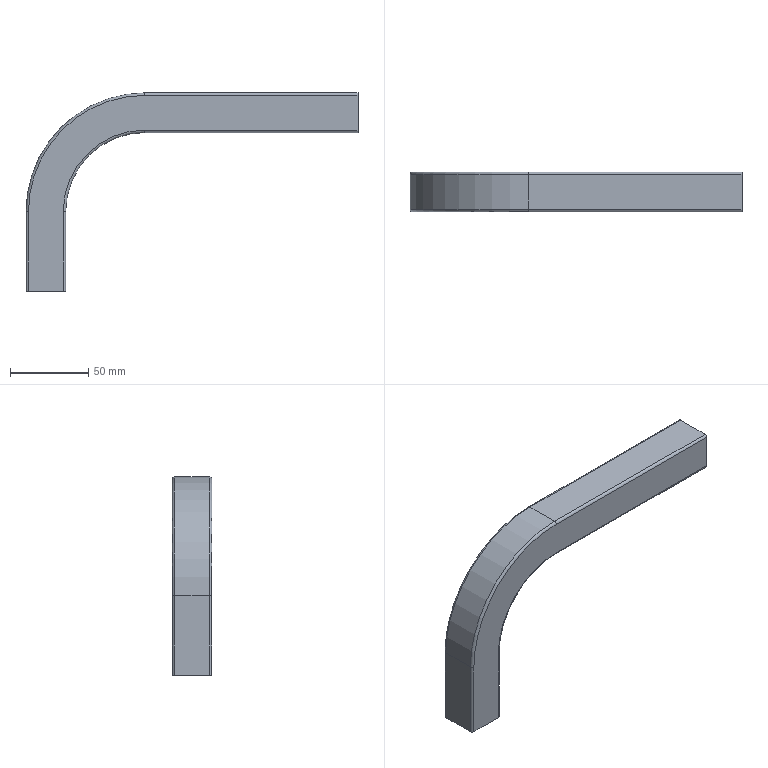Part | NX | features BREP 1 | 1 solid | 30 faces | box 212.725 x 25.4 x 127 mm | volume 52656 mm3 | plane 14 | cylinder 12 | torus 4 | commonest cylinder face diameters 3.175 x8 101.6 x1 105.562 x1 148.438 x1 152.4 x1
STEP:
#1=CARTESIAN_POINT('',(11.113,12.7,-114.3));
#2=VERTEX_POINT('',#1);
#3=CARTESIAN_POINT('',(-11.113,12.7,-114.3));
#4=VERTEX_POINT('',#3);
#5=CARTESIAN_POINT('',(11.113,12.7,-114.3));
#6=DIRECTION('',(-1.,0.,0.));
#7=VECTOR('',#6,1000.);
#8=LINE('',#5,#7);
#9=EDGE_CURVE('',#2,#4,#8,.T.);
#10=ORIENTED_EDGE('',*,*,#9,.F.);
#11=CARTESIAN_POINT('',(12.7,11.113,-114.3));
#12=VERTEX_POINT('',#11);
#13=CARTESIAN_POINT('',(11.113,11.113,-114.3));
#14=DIRECTION('',(0.,0.,-1.));
#15=DIRECTION('',(0.,1.,0.));
#16=AXIS2_PLACEMENT_3D('',#13,#14,#15);
#17=CIRCLE('',#16,1.587);
#18=EDGE_CURVE('',#2,#12,#17,.T.);
#19=ORIENTED_EDGE('',*,*,#18,.T.);
#20=CARTESIAN_POINT('',(12.7,-11.113,-114.3));
#21=VERTEX_POINT('',#20);
#22=CARTESIAN_POINT('',(12.7,-11.113,-114.3));
#23=DIRECTION('',(0.,1.,0.));
#24=VECTOR('',#23,1000.);
#25=LINE('',#22,#24);
#26=EDGE_CURVE('',#21,#12,#25,.T.);
#27=ORIENTED_EDGE('',*,*,#26,.F.);
#28=CARTESIAN_POINT('',(11.113,-12.7,-114.3));
#29=VERTEX_POINT('',#28);
#30=CARTESIAN_POINT('',(11.113,-11.113,-114.3));
#31=DIRECTION('',(0.,0.,-1.));
#32=DIRECTION('',(1.,0.,0.));
#33=AXIS2_PLACEMENT_3D('',#30,#31,#32);
#34=CIRCLE('',#33,1.587);
#35=EDGE_CURVE('',#21,#29,#34,.T.);
#36=ORIENTED_EDGE('',*,*,#35,.T.);
#37=CARTESIAN_POINT('',(-11.113,-12.7,-114.3));
#38=VERTEX_POINT('',#37);
#39=CARTESIAN_POINT('',(-11.113,-12.7,-114.3));
#40=DIRECTION('',(1.,0.,0.));
#41=VECTOR('',#40,1000.);
#42=LINE('',#39,#41);
#43=EDGE_CURVE('',#38,#29,#42,.T.);
#44=ORIENTED_EDGE('',*,*,#43,.F.);
#45=CARTESIAN_POINT('',(-12.7,-11.113,-114.3));
#46=VERTEX_POINT('',#45);
#47=CARTESIAN_POINT('',(-11.113,-11.113,-114.3));
#48=DIRECTION('',(0.,0.,-1.));
#49=DIRECTION('',(0.,-1.,0.));
#50=AXIS2_PLACEMENT_3D('',#47,#48,#49);
#51=CIRCLE('',#50,1.587);
#52=EDGE_CURVE('',#38,#46,#51,.T.);
#53=ORIENTED_EDGE('',*,*,#52,.T.);
#54=CARTESIAN_POINT('',(-12.7,11.113,-114.3));
#55=VERTEX_POINT('',#54);
#56=CARTESIAN_POINT('',(-12.7,11.113,-114.3));
#57=DIRECTION('',(0.,-1.,0.));
#58=VECTOR('',#57,1000.);
#59=LINE('',#56,#58);
#60=EDGE_CURVE('',#55,#46,#59,.T.);
#61=ORIENTED_EDGE('',*,*,#60,.F.);
#62=CARTESIAN_POINT('',(-11.113,11.113,-114.3));
#63=DIRECTION('',(0.,0.,-1.));
#64=DIRECTION('',(-1.,0.,0.));
#65=AXIS2_PLACEMENT_3D('',#62,#63,#64);
#66=CIRCLE('',#65,1.587);
#67=EDGE_CURVE('',#55,#4,#66,.T.);
#68=ORIENTED_EDGE('',*,*,#67,.T.);
#69=EDGE_LOOP('',(#10,#19,#27,#36,#44,#53,#61,#68));
#70=FACE_BOUND('',#69,.T.);
#71=CARTESIAN_POINT('',(-10.719,-10.719,-114.3));
#72=VERTEX_POINT('',#71);
#73=CARTESIAN_POINT('',(-10.719,10.719,-114.3));
#74=VERTEX_POINT('',#73);
#75=CARTESIAN_POINT('',(-10.719,-10.719,-114.3));
#76=DIRECTION('',(0.,1.,0.));
#77=VECTOR('',#76,1000.);
#78=LINE('',#75,#77);
#79=EDGE_CURVE('',#72,#74,#78,.T.);
#80=ORIENTED_EDGE('',*,*,#79,.F.);
#81=CARTESIAN_POINT('',(10.719,-10.719,-114.3));
#82=VERTEX_POINT('',#81);
#83=CARTESIAN_POINT('',(10.719,-10.719,-114.3));
#84=DIRECTION('',(-1.,0.,0.));
#85=VECTOR('',#84,1000.);
#86=LINE('',#83,#85);
#87=EDGE_CURVE('',#82,#72,#86,.T.);
#88=ORIENTED_EDGE('',*,*,#87,.F.);
#89=CARTESIAN_POINT('',(10.719,10.719,-114.3));
#90=VERTEX_POINT('',#89);
#91=CARTESIAN_POINT('',(10.719,10.719,-114.3));
#92=DIRECTION('',(0.,-1.,0.));
#93=VECTOR('',#92,1000.);
#94=LINE('',#91,#93);
#95=EDGE_CURVE('',#90,#82,#94,.T.);
#96=ORIENTED_EDGE('',*,*,#95,.F.);
#97=CARTESIAN_POINT('',(-10.719,10.719,-114.3));
#98=DIRECTION('',(1.,0.,0.));
#99=VECTOR('',#98,1000.);
#100=LINE('',#97,#99);
#101=EDGE_CURVE('',#74,#90,#100,.T.);
#102=ORIENTED_EDGE('',*,*,#101,.F.);
#103=EDGE_LOOP('',(#80,#88,#96,#102));
#104=FACE_BOUND('',#103,.T.);
#105=CARTESIAN_POINT('',(0.,0.,-114.3));
#106=DIRECTION('',(0.,0.,1.));
#107=DIRECTION('',(1.,0.,0.));
#108=AXIS2_PLACEMENT_3D('',#105,#106,#107);
#109=PLANE('',#108);
#110=ADVANCED_FACE('',(#70,#104),#109,.F.);
#111=CARTESIAN_POINT('',(10.719,10.719,-63.5));
#112=VERTEX_POINT('',#111);
#113=CARTESIAN_POINT('',(10.719,10.719,-114.3));
#114=DIRECTION('',(0.,0.,1.));
#115=VECTOR('',#114,1000.);
#116=LINE('',#113,#115);
#117=EDGE_CURVE('',#90,#112,#116,.T.);
#118=ORIENTED_EDGE('',*,*,#117,.T.);
#119=CARTESIAN_POINT('',(63.5,10.719,-10.719));
#120=VERTEX_POINT('',#119);
#121=CARTESIAN_POINT('',(63.5,10.719,-63.5));
#122=DIRECTION('',(0.,1.,0.));
#123=DIRECTION('',(-1.,0.,0.));
#124=AXIS2_PLACEMENT_3D('',#121,#122,#123);
#125=CIRCLE('',#124,52.781);
#126=EDGE_CURVE('',#112,#120,#125,.T.);
#127=ORIENTED_EDGE('',*,*,#126,.T.);
#128=CARTESIAN_POINT('',(200.025,10.719,-10.719));
#129=VERTEX_POINT('',#128);
#130=CARTESIAN_POINT('',(63.5,10.719,-10.719));
#131=DIRECTION('',(1.,0.,0.));
#132=VECTOR('',#131,1000.);
#133=LINE('',#130,#132);
#134=EDGE_CURVE('',#120,#129,#133,.T.);
#135=ORIENTED_EDGE('',*,*,#134,.T.);
#136=CARTESIAN_POINT('',(200.025,10.719,10.719));
#137=VERTEX_POINT('',#136);
#138=CARTESIAN_POINT('',(200.025,10.719,10.719));
#139=DIRECTION('',(0.,0.,-1.));
#140=VECTOR('',#139,1000.);
#141=LINE('',#138,#140);
#142=EDGE_CURVE('',#137,#129,#141,.T.);
#143=ORIENTED_EDGE('',*,*,#142,.F.);
#144=CARTESIAN_POINT('',(63.5,10.719,10.719));
#145=VERTEX_POINT('',#144);
#146=CARTESIAN_POINT('',(63.5,10.719,10.719));
#147=DIRECTION('',(1.,0.,0.));
#148=VECTOR('',#147,1000.);
#149=LINE('',#146,#148);
#150=EDGE_CURVE('',#145,#137,#149,.T.);
#151=ORIENTED_EDGE('',*,*,#150,.F.);
#152=CARTESIAN_POINT('',(-10.719,10.719,-63.5));
#153=VERTEX_POINT('',#152);
#154=CARTESIAN_POINT('',(63.5,10.719,-63.5));
#155=DIRECTION('',(0.,1.,0.));
#156=DIRECTION('',(-1.,0.,0.));
#157=AXIS2_PLACEMENT_3D('',#154,#155,#156);
#158=CIRCLE('',#157,74.219);
#159=EDGE_CURVE('',#153,#145,#158,.T.);
#160=ORIENTED_EDGE('',*,*,#159,.F.);
#161=CARTESIAN_POINT('',(-10.719,10.719,-114.3));
#162=DIRECTION('',(0.,0.,1.));
#163=VECTOR('',#162,1000.);
#164=LINE('',#161,#163);
#165=EDGE_CURVE('',#74,#153,#164,.T.);
#166=ORIENTED_EDGE('',*,*,#165,.F.);
#167=ORIENTED_EDGE('',*,*,#101,.T.);
#168=EDGE_LOOP('',(#118,#127,#135,#143,#151,#160,#166,#167));
#169=FACE_BOUND('',#168,.T.);
#170=CARTESIAN_POINT('',(-10.719,10.719,-114.3));
#171=DIRECTION('',(0.,-1.,0.));
#172=DIRECTION('',(0.,0.,-1.));
#173=AXIS2_PLACEMENT_3D('',#170,#171,#172);
#174=PLANE('',#173);
#175=ADVANCED_FACE('',(#169),#174,.T.);
#176=ORIENTED_EDGE('',*,*,#165,.T.);
#177=CARTESIAN_POINT('',(-10.719,-10.719,-63.5));
#178=VERTEX_POINT('',#177);
#179=CARTESIAN_POINT('',(-10.719,-10.719,-63.5));
#180=DIRECTION('',(0.,1.,0.));
#181=VECTOR('',#180,1000.);
#182=LINE('',#179,#181);
#183=EDGE_CURVE('',#178,#153,#182,.T.);
#184=ORIENTED_EDGE('',*,*,#183,.F.);
#185=CARTESIAN_POINT('',(-10.719,-10.719,-114.3));
#186=DIRECTION('',(0.,0.,1.));
#187=VECTOR('',#186,1000.);
#188=LINE('',#185,#187);
#189=EDGE_CURVE('',#72,#178,#188,.T.);
#190=ORIENTED_EDGE('',*,*,#189,.F.);
#191=ORIENTED_EDGE('',*,*,#79,.T.);
#192=EDGE_LOOP('',(#176,#184,#190,#191));
#193=FACE_BOUND('',#192,.T.);
#194=CARTESIAN_POINT('',(-10.719,-10.719,-114.3));
#195=DIRECTION('',(1.,0.,0.));
#196=DIRECTION('',(0.,1.,0.));
#197=AXIS2_PLACEMENT_3D('',#194,#195,#196);
#198=PLANE('',#197);
#199=ADVANCED_FACE('',(#193),#198,.T.);
#200=ORIENTED_EDGE('',*,*,#189,.T.);
#201=CARTESIAN_POINT('',(63.5,-10.719,10.719));
#202=VERTEX_POINT('',#201);
#203=CARTESIAN_POINT('',(63.5,-10.719,-63.5));
#204=DIRECTION('',(0.,1.,0.));
#205=DIRECTION('',(-1.,0.,0.));
#206=AXIS2_PLACEMENT_3D('',#203,#204,#205);
#207=CIRCLE('',#206,74.219);
#208=EDGE_CURVE('',#178,#202,#207,.T.);
#209=ORIENTED_EDGE('',*,*,#208,.T.);
#210=CARTESIAN_POINT('',(200.025,-10.719,10.719));
#211=VERTEX_POINT('',#210);
#212=CARTESIAN_POINT('',(63.5,-10.719,10.719));
#213=DIRECTION('',(1.,0.,0.));
#214=VECTOR('',#213,1000.);
#215=LINE('',#212,#214);
#216=EDGE_CURVE('',#202,#211,#215,.T.);
#217=ORIENTED_EDGE('',*,*,#216,.T.);
#218=CARTESIAN_POINT('',(200.025,-10.719,-10.719));
#219=VERTEX_POINT('',#218);
#220=CARTESIAN_POINT('',(200.025,-10.719,-10.719));
#221=DIRECTION('',(0.,0.,1.));
#222=VECTOR('',#221,1000.);
#223=LINE('',#220,#222);
#224=EDGE_CURVE('',#219,#211,#223,.T.);
#225=ORIENTED_EDGE('',*,*,#224,.F.);
#226=CARTESIAN_POINT('',(63.5,-10.719,-10.719));
#227=VERTEX_POINT('',#226);
#228=CARTESIAN_POINT('',(63.5,-10.719,-10.719));
#229=DIRECTION('',(1.,0.,0.));
#230=VECTOR('',#229,1000.);
#231=LINE('',#228,#230);
#232=EDGE_CURVE('',#227,#219,#231,.T.);
#233=ORIENTED_EDGE('',*,*,#232,.F.);
#234=CARTESIAN_POINT('',(10.719,-10.719,-63.5));
#235=VERTEX_POINT('',#234);
#236=CARTESIAN_POINT('',(63.5,-10.719,-63.5));
#237=DIRECTION('',(0.,1.,0.));
#238=DIRECTION('',(-1.,0.,0.));
#239=AXIS2_PLACEMENT_3D('',#236,#237,#238);
#240=CIRCLE('',#239,52.781);
#241=EDGE_CURVE('',#235,#227,#240,.T.);
#242=ORIENTED_EDGE('',*,*,#241,.F.);
#243=CARTESIAN_POINT('',(10.719,-10.719,-114.3));
#244=DIRECTION('',(0.,0.,1.));
#245=VECTOR('',#244,1000.);
#246=LINE('',#243,#245);
#247=EDGE_CURVE('',#82,#235,#246,.T.);
#248=ORIENTED_EDGE('',*,*,#247,.F.);
#249=ORIENTED_EDGE('',*,*,#87,.T.);
#250=EDGE_LOOP('',(#200,#209,#217,#225,#233,#242,#248,#249));
#251=FACE_BOUND('',#250,.T.);
#252=CARTESIAN_POINT('',(10.719,-10.719,-114.3));
#253=DIRECTION('',(0.,1.,0.));
#254=DIRECTION('',(1.,0.,0.));
#255=AXIS2_PLACEMENT_3D('',#252,#253,#254);
#256=PLANE('',#255);
#257=ADVANCED_FACE('',(#251),#256,.T.);
#258=ORIENTED_EDGE('',*,*,#247,.T.);
#259=CARTESIAN_POINT('',(10.719,10.719,-63.5));
#260=DIRECTION('',(0.,-1.,0.));
#261=VECTOR('',#260,1000.);
#262=LINE('',#259,#261);
#263=EDGE_CURVE('',#112,#235,#262,.T.);
#264=ORIENTED_EDGE('',*,*,#263,.F.);
#265=ORIENTED_EDGE('',*,*,#117,.F.);
#266=ORIENTED_EDGE('',*,*,#95,.T.);
#267=EDGE_LOOP('',(#258,#264,#265,#266));
#268=FACE_BOUND('',#267,.T.);
#269=CARTESIAN_POINT('',(10.719,10.719,-114.3));
#270=DIRECTION('',(-1.,0.,0.));
#271=DIRECTION('',(0.,0.,1.));
#272=AXIS2_PLACEMENT_3D('',#269,#270,#271);
#273=PLANE('',#272);
#274=ADVANCED_FACE('',(#268),#273,.T.);
#275=ORIENTED_EDGE('',*,*,#241,.T.);
#276=CARTESIAN_POINT('',(63.5,10.719,-10.719));
#277=DIRECTION('',(0.,-1.,0.));
#278=VECTOR('',#277,1000.);
#279=LINE('',#276,#278);
#280=EDGE_CURVE('',#120,#227,#279,.T.);
#281=ORIENTED_EDGE('',*,*,#280,.F.);
#282=ORIENTED_EDGE('',*,*,#126,.F.);
#283=ORIENTED_EDGE('',*,*,#263,.T.);
#284=EDGE_LOOP('',(#275,#281,#282,#283));
#285=FACE_BOUND('',#284,.T.);
#286=CARTESIAN_POINT('',(63.5,-25.4,-63.5));
#287=DIRECTION('',(0.,1.,0.));
#288=DIRECTION('',(1.,0.,0.));
#289=AXIS2_PLACEMENT_3D('',#286,#287,#288);
#290=CYLINDRICAL_SURFACE('',#289,52.781);
#291=ADVANCED_FACE('',(#285),#290,.T.);
#292=ORIENTED_EDGE('',*,*,#232,.T.);
#293=CARTESIAN_POINT('',(200.025,10.719,-10.719));
#294=DIRECTION('',(0.,-1.,0.));
#295=VECTOR('',#294,1000.);
#296=LINE('',#293,#295);
#297=EDGE_CURVE('',#129,#219,#296,.T.);
#298=ORIENTED_EDGE('',*,*,#297,.F.);
#299=ORIENTED_EDGE('',*,*,#134,.F.);
#300=ORIENTED_EDGE('',*,*,#280,.T.);
#301=EDGE_LOOP('',(#292,#298,#299,#300));
#302=FACE_BOUND('',#301,.T.);
#303=CARTESIAN_POINT('',(63.5,10.719,-10.719));
#304=DIRECTION('',(0.,0.,1.));
#305=DIRECTION('',(1.,0.,0.));
#306=AXIS2_PLACEMENT_3D('',#303,#304,#305);
#307=PLANE('',#306);
#308=ADVANCED_FACE('',(#302),#307,.T.);
#309=CARTESIAN_POINT('',(200.025,11.113,12.7));
#310=VERTEX_POINT('',#309);
#311=CARTESIAN_POINT('',(200.025,-11.113,12.7));
#312=VERTEX_POINT('',#311);
#313=CARTESIAN_POINT('',(200.025,11.113,12.7));
#314=DIRECTION('',(0.,-1.,0.));
#315=VECTOR('',#314,1000.);
#316=LINE('',#313,#315);
#317=EDGE_CURVE('',#310,#312,#316,.T.);
#318=ORIENTED_EDGE('',*,*,#317,.T.);
#319=CARTESIAN_POINT('',(200.025,-12.7,11.113));
#320=VERTEX_POINT('',#319);
#321=CARTESIAN_POINT('',(200.025,-11.113,11.113));
#322=DIRECTION('',(1.,0.,0.));
#323=DIRECTION('',(0.,0.,1.));
#324=AXIS2_PLACEMENT_3D('',#321,#322,#323);
#325=CIRCLE('',#324,1.587);
#326=EDGE_CURVE('',#312,#320,#325,.T.);
#327=ORIENTED_EDGE('',*,*,#326,.T.);
#328=CARTESIAN_POINT('',(200.025,-12.7,-11.113));
#329=VERTEX_POINT('',#328);
#330=CARTESIAN_POINT('',(200.025,-12.7,11.113));
#331=DIRECTION('',(0.,0.,-1.));
#332=VECTOR('',#331,1000.);
#333=LINE('',#330,#332);
#334=EDGE_CURVE('',#320,#329,#333,.T.);
#335=ORIENTED_EDGE('',*,*,#334,.T.);
#336=CARTESIAN_POINT('',(200.025,-11.113,-12.7));
#337=VERTEX_POINT('',#336);
#338=CARTESIAN_POINT('',(200.025,-11.113,-11.113));
#339=DIRECTION('',(1.,0.,0.));
#340=DIRECTION('',(0.,-1.,0.));
#341=AXIS2_PLACEMENT_3D('',#338,#339,#340);
#342=CIRCLE('',#341,1.587);
#343=EDGE_CURVE('',#329,#337,#342,.T.);
#344=ORIENTED_EDGE('',*,*,#343,.T.);
#345=CARTESIAN_POINT('',(200.025,11.113,-12.7));
#346=VERTEX_POINT('',#345);
#347=CARTESIAN_POINT('',(200.025,-11.113,-12.7));
#348=DIRECTION('',(0.,1.,0.));
#349=VECTOR('',#348,1000.);
#350=LINE('',#347,#349);
#351=EDGE_CURVE('',#337,#346,#350,.T.);
#352=ORIENTED_EDGE('',*,*,#351,.T.);
#353=CARTESIAN_POINT('',(200.025,12.7,-11.113));
#354=VERTEX_POINT('',#353);
#355=CARTESIAN_POINT('',(200.025,11.113,-11.113));
#356=DIRECTION('',(1.,0.,0.));
#357=DIRECTION('',(0.,0.,-1.));
#358=AXIS2_PLACEMENT_3D('',#355,#356,#357);
#359=CIRCLE('',#358,1.587);
#360=EDGE_CURVE('',#346,#354,#359,.T.);
#361=ORIENTED_EDGE('',*,*,#360,.T.);
#362=CARTESIAN_POINT('',(200.025,12.7,11.113));
#363=VERTEX_POINT('',#362);
#364=CARTESIAN_POINT('',(200.025,12.7,-11.113));
#365=DIRECTION('',(0.,0.,1.));
#366=VECTOR('',#365,1000.);
#367=LINE('',#364,#366);
#368=EDGE_CURVE('',#354,#363,#367,.T.);
#369=ORIENTED_EDGE('',*,*,#368,.T.);
#370=CARTESIAN_POINT('',(200.025,11.113,11.113));
#371=DIRECTION('',(1.,0.,0.));
#372=DIRECTION('',(0.,1.,0.));
#373=AXIS2_PLACEMENT_3D('',#370,#371,#372);
#374=CIRCLE('',#373,1.587);
#375=EDGE_CURVE('',#363,#310,#374,.T.);
#376=ORIENTED_EDGE('',*,*,#375,.T.);
#377=EDGE_LOOP('',(#318,#327,#335,#344,#352,#361,#369,#376));
#378=FACE_BOUND('',#377,.T.);
#379=ORIENTED_EDGE('',*,*,#297,.T.);
#380=ORIENTED_EDGE('',*,*,#224,.T.);
#381=CARTESIAN_POINT('',(200.025,-10.719,10.719));
#382=DIRECTION('',(0.,1.,0.));
#383=VECTOR('',#382,1000.);
#384=LINE('',#381,#383);
#385=EDGE_CURVE('',#211,#137,#384,.T.);
#386=ORIENTED_EDGE('',*,*,#385,.T.);
#387=ORIENTED_EDGE('',*,*,#142,.T.);
#388=EDGE_LOOP('',(#379,#380,#386,#387));
#389=FACE_BOUND('',#388,.T.);
#390=CARTESIAN_POINT('',(200.025,0.,0.));
#391=DIRECTION('',(1.,0.,0.));
#392=DIRECTION('',(0.,1.,0.));
#393=AXIS2_PLACEMENT_3D('',#390,#391,#392);
#394=PLANE('',#393);
#395=ADVANCED_FACE('',(#378,#389),#394,.T.);
#396=ORIENTED_EDGE('',*,*,#150,.T.);
#397=ORIENTED_EDGE('',*,*,#385,.F.);
#398=ORIENTED_EDGE('',*,*,#216,.F.);
#399=CARTESIAN_POINT('',(63.5,-10.719,10.719));
#400=DIRECTION('',(0.,1.,0.));
#401=VECTOR('',#400,1000.);
#402=LINE('',#399,#401);
#403=EDGE_CURVE('',#202,#145,#402,.T.);
#404=ORIENTED_EDGE('',*,*,#403,.T.);
#405=EDGE_LOOP('',(#396,#397,#398,#404));
#406=FACE_BOUND('',#405,.T.);
#407=CARTESIAN_POINT('',(63.5,-10.719,10.719));
#408=DIRECTION('',(0.,0.,-1.));
#409=DIRECTION('',(0.,-1.,0.));
#410=AXIS2_PLACEMENT_3D('',#407,#408,#409);
#411=PLANE('',#410);
#412=ADVANCED_FACE('',(#406),#411,.T.);
#413=ORIENTED_EDGE('',*,*,#159,.T.);
#414=ORIENTED_EDGE('',*,*,#403,.F.);
#415=ORIENTED_EDGE('',*,*,#208,.F.);
#416=ORIENTED_EDGE('',*,*,#183,.T.);
#417=EDGE_LOOP('',(#413,#414,#415,#416));
#418=FACE_BOUND('',#417,.T.);
#419=CARTESIAN_POINT('',(63.5,-25.4,-63.5));
#420=DIRECTION('',(0.,1.,0.));
#421=DIRECTION('',(1.,0.,0.));
#422=AXIS2_PLACEMENT_3D('',#419,#420,#421);
#423=CYLINDRICAL_SURFACE('',#422,74.219);
#424=ADVANCED_FACE('',(#418),#423,.F.);
#425=ORIENTED_EDGE('',*,*,#375,.F.);
#426=CARTESIAN_POINT('',(63.5,12.7,11.112));
#427=VERTEX_POINT('',#426);
#428=CARTESIAN_POINT('',(200.025,12.7,11.113));
#429=DIRECTION('',(-1.,0.,0.));
#430=VECTOR('',#429,1000.);
#431=LINE('',#428,#430);
#432=EDGE_CURVE('',#363,#427,#431,.T.);
#433=ORIENTED_EDGE('',*,*,#432,.T.);
#434=CARTESIAN_POINT('',(63.5,11.113,12.7));
#435=VERTEX_POINT('',#434);
#436=CARTESIAN_POINT('',(63.5,11.113,11.113));
#437=DIRECTION('',(-1.,0.,0.));
#438=DIRECTION('',(0.,0.,1.));
#439=AXIS2_PLACEMENT_3D('',#436,#437,#438);
#440=CIRCLE('',#439,1.587);
#441=EDGE_CURVE('',#435,#427,#440,.T.);
#442=ORIENTED_EDGE('',*,*,#441,.F.);
#443=CARTESIAN_POINT('',(200.025,11.113,12.7));
#444=DIRECTION('',(-1.,0.,0.));
#445=VECTOR('',#444,1000.);
#446=LINE('',#443,#445);
#447=EDGE_CURVE('',#310,#435,#446,.T.);
#448=ORIENTED_EDGE('',*,*,#447,.F.);
#449=EDGE_LOOP('',(#425,#433,#442,#448));
#450=FACE_BOUND('',#449,.T.);
#451=CARTESIAN_POINT('',(200.408,11.113,11.113));
#452=DIRECTION('',(-1.,0.,0.));
#453=DIRECTION('',(0.,0.,1.));
#454=AXIS2_PLACEMENT_3D('',#451,#452,#453);
#455=CYLINDRICAL_SURFACE('',#454,1.587);
#456=ADVANCED_FACE('',(#450),#455,.T.);
#457=CARTESIAN_POINT('',(63.5,-11.113,12.7));
#458=VERTEX_POINT('',#457);
#459=CARTESIAN_POINT('',(63.5,11.113,12.7));
#460=DIRECTION('',(0.,-1.,0.));
#461=VECTOR('',#460,1000.);
#462=LINE('',#459,#461);
#463=EDGE_CURVE('',#435,#458,#462,.T.);
#464=ORIENTED_EDGE('',*,*,#463,.T.);
#465=CARTESIAN_POINT('',(200.025,-11.113,12.7));
#466=DIRECTION('',(-1.,0.,0.));
#467=VECTOR('',#466,1000.);
#468=LINE('',#465,#467);
#469=EDGE_CURVE('',#312,#458,#468,.T.);
#470=ORIENTED_EDGE('',*,*,#469,.F.);
#471=ORIENTED_EDGE('',*,*,#317,.F.);
#472=ORIENTED_EDGE('',*,*,#447,.T.);
#473=EDGE_LOOP('',(#464,#470,#471,#472));
#474=FACE_BOUND('',#473,.T.);
#475=CARTESIAN_POINT('',(63.5,12.7,12.7));
#476=DIRECTION('',(0.,0.,1.));
#477=DIRECTION('',(1.,0.,0.));
#478=AXIS2_PLACEMENT_3D('',#475,#476,#477);
#479=PLANE('',#478);
#480=ADVANCED_FACE('',(#474),#479,.T.);
#481=ORIENTED_EDGE('',*,*,#326,.F.);
#482=ORIENTED_EDGE('',*,*,#469,.T.);
#483=CARTESIAN_POINT('',(63.5,-12.7,11.112));
#484=VERTEX_POINT('',#483);
#485=CARTESIAN_POINT('',(63.5,-11.113,11.113));
#486=DIRECTION('',(-1.,0.,0.));
#487=DIRECTION('',(0.,-1.,0.));
#488=AXIS2_PLACEMENT_3D('',#485,#486,#487);
#489=CIRCLE('',#488,1.587);
#490=EDGE_CURVE('',#484,#458,#489,.T.);
#491=ORIENTED_EDGE('',*,*,#490,.F.);
#492=CARTESIAN_POINT('',(200.025,-12.7,11.113));
#493=DIRECTION('',(-1.,0.,0.));
#494=VECTOR('',#493,1000.);
#495=LINE('',#492,#494);
#496=EDGE_CURVE('',#320,#484,#495,.T.);
#497=ORIENTED_EDGE('',*,*,#496,.F.);
#498=EDGE_LOOP('',(#481,#482,#491,#497));
#499=FACE_BOUND('',#498,.T.);
#500=CARTESIAN_POINT('',(200.393,-11.113,11.113));
#501=DIRECTION('',(-1.,0.,0.));
#502=DIRECTION('',(0.,-1.,0.));
#503=AXIS2_PLACEMENT_3D('',#500,#501,#502);
#504=CYLINDRICAL_SURFACE('',#503,1.587);
#505=ADVANCED_FACE('',(#499),#504,.T.);
#506=ORIENTED_EDGE('',*,*,#43,.T.);
#507=CARTESIAN_POINT('',(11.113,-12.7,-63.5));
#508=VERTEX_POINT('',#507);
#509=CARTESIAN_POINT('',(11.113,-12.7,-63.5));
#510=DIRECTION('',(0.,0.,-1.));
#511=VECTOR('',#510,1000.);
#512=LINE('',#509,#511);
#513=EDGE_CURVE('',#508,#29,#512,.T.);
#514=ORIENTED_EDGE('',*,*,#513,.F.);
#515=CARTESIAN_POINT('',(63.5,-12.7,-11.113));
#516=VERTEX_POINT('',#515);
#517=CARTESIAN_POINT('',(63.5,-12.7,-63.5));
#518=DIRECTION('',(0.,-1.,0.));
#519=DIRECTION('',(0.,0.,1.));
#520=AXIS2_PLACEMENT_3D('',#517,#518,#519);
#521=CIRCLE('',#520,52.387);
#522=EDGE_CURVE('',#516,#508,#521,.T.);
#523=ORIENTED_EDGE('',*,*,#522,.F.);
#524=CARTESIAN_POINT('',(200.025,-12.7,-11.113));
#525=DIRECTION('',(-1.,0.,0.));
#526=VECTOR('',#525,1000.);
#527=LINE('',#524,#526);
#528=EDGE_CURVE('',#329,#516,#527,.T.);
#529=ORIENTED_EDGE('',*,*,#528,.F.);
#530=ORIENTED_EDGE('',*,*,#334,.F.);
#531=ORIENTED_EDGE('',*,*,#496,.T.);
#532=CARTESIAN_POINT('',(-11.113,-12.7,-63.5));
#533=VERTEX_POINT('',#532);
#534=CARTESIAN_POINT('',(63.5,-12.7,-63.5));
#535=DIRECTION('',(0.,-1.,0.));
#536=DIRECTION('',(0.,0.,1.));
#537=AXIS2_PLACEMENT_3D('',#534,#535,#536);
#538=CIRCLE('',#537,74.612);
#539=EDGE_CURVE('',#484,#533,#538,.T.);
#540=ORIENTED_EDGE('',*,*,#539,.T.);
#541=CARTESIAN_POINT('',(-11.113,-12.7,-63.5));
#542=DIRECTION('',(0.,0.,-1.));
#543=VECTOR('',#542,1000.);
#544=LINE('',#541,#543);
#545=EDGE_CURVE('',#533,#38,#544,.T.);
#546=ORIENTED_EDGE('',*,*,#545,.T.);
#547=EDGE_LOOP('',(#506,#514,#523,#529,#530,#531,#540,#546));
#548=FACE_BOUND('',#547,.T.);
#549=CARTESIAN_POINT('',(-12.7,-12.7,-114.3));
#550=DIRECTION('',(0.,-1.,0.));
#551=DIRECTION('',(0.,0.,-1.));
#552=AXIS2_PLACEMENT_3D('',#549,#550,#551);
#553=PLANE('',#552);
#554=ADVANCED_FACE('',(#548),#553,.T.);
#555=CARTESIAN_POINT('',(-12.7,-11.113,-63.5));
#556=VERTEX_POINT('',#555);
#557=CARTESIAN_POINT('',(-11.113,-11.113,-63.5));
#558=DIRECTION('',(0.,0.,-1.));
#559=DIRECTION('',(0.,-1.,0.));
#560=AXIS2_PLACEMENT_3D('',#557,#558,#559);
#561=CIRCLE('',#560,1.587);
#562=EDGE_CURVE('',#533,#556,#561,.T.);
#563=ORIENTED_EDGE('',*,*,#562,.T.);
#564=CARTESIAN_POINT('',(-12.7,-11.113,-63.5));
#565=DIRECTION('',(0.,0.,-1.));
#566=VECTOR('',#565,1000.);
#567=LINE('',#564,#566);
#568=EDGE_CURVE('',#556,#46,#567,.T.);
#569=ORIENTED_EDGE('',*,*,#568,.T.);
#570=ORIENTED_EDGE('',*,*,#52,.F.);
#571=ORIENTED_EDGE('',*,*,#545,.F.);
#572=EDGE_LOOP('',(#563,#569,#570,#571));
#573=FACE_BOUND('',#572,.T.);
#574=CARTESIAN_POINT('',(-11.113,-11.113,-62.925));
#575=DIRECTION('',(0.,0.,-1.));
#576=DIRECTION('',(0.,-1.,0.));
#577=AXIS2_PLACEMENT_3D('',#574,#575,#576);
#578=CYLINDRICAL_SURFACE('',#577,1.587);
#579=ADVANCED_FACE('',(#573),#578,.T.);
#580=ORIENTED_EDGE('',*,*,#60,.T.);
#581=ORIENTED_EDGE('',*,*,#568,.F.);
#582=CARTESIAN_POINT('',(-12.7,11.113,-63.5));
#583=VERTEX_POINT('',#582);
#584=CARTESIAN_POINT('',(-12.7,11.113,-63.5));
#585=DIRECTION('',(0.,-1.,0.));
#586=VECTOR('',#585,1000.);
#587=LINE('',#584,#586);
#588=EDGE_CURVE('',#583,#556,#587,.T.);
#589=ORIENTED_EDGE('',*,*,#588,.F.);
#590=CARTESIAN_POINT('',(-12.7,11.113,-63.5));
#591=DIRECTION('',(0.,0.,-1.));
#592=VECTOR('',#591,1000.);
#593=LINE('',#590,#592);
#594=EDGE_CURVE('',#583,#55,#593,.T.);
#595=ORIENTED_EDGE('',*,*,#594,.T.);
#596=EDGE_LOOP('',(#580,#581,#589,#595));
#597=FACE_BOUND('',#596,.T.);
#598=CARTESIAN_POINT('',(-12.7,12.7,-114.3));
#599=DIRECTION('',(-1.,0.,0.));
#600=DIRECTION('',(0.,0.,1.));
#601=AXIS2_PLACEMENT_3D('',#598,#599,#600);
#602=PLANE('',#601);
#603=ADVANCED_FACE('',(#597),#602,.T.);
#604=CARTESIAN_POINT('',(-11.113,12.7,-63.5));
#605=VERTEX_POINT('',#604);
#606=CARTESIAN_POINT('',(-11.113,11.113,-63.5));
#607=DIRECTION('',(0.,0.,-1.));
#608=DIRECTION('',(-1.,0.,0.));
#609=AXIS2_PLACEMENT_3D('',#606,#607,#608);
#610=CIRCLE('',#609,1.587);
#611=EDGE_CURVE('',#583,#605,#610,.T.);
#612=ORIENTED_EDGE('',*,*,#611,.T.);
#613=CARTESIAN_POINT('',(-11.113,12.7,-63.5));
#614=DIRECTION('',(0.,0.,-1.));
#615=VECTOR('',#614,1000.);
#616=LINE('',#613,#615);
#617=EDGE_CURVE('',#605,#4,#616,.T.);
#618=ORIENTED_EDGE('',*,*,#617,.T.);
#619=ORIENTED_EDGE('',*,*,#67,.F.);
#620=ORIENTED_EDGE('',*,*,#594,.F.);
#621=EDGE_LOOP('',(#612,#618,#619,#620));
#622=FACE_BOUND('',#621,.T.);
#623=CARTESIAN_POINT('',(-11.113,11.113,-63.11));
#624=DIRECTION('',(0.,0.,-1.));
#625=DIRECTION('',(-1.,0.,0.));
#626=AXIS2_PLACEMENT_3D('',#623,#624,#625);
#627=CYLINDRICAL_SURFACE('',#626,1.587);
#628=ADVANCED_FACE('',(#622),#627,.T.);
#629=CARTESIAN_POINT('',(63.5,12.7,-63.5));
#630=DIRECTION('',(0.,-1.,0.));
#631=DIRECTION('',(0.,0.,1.));
#632=AXIS2_PLACEMENT_3D('',#629,#630,#631);
#633=CIRCLE('',#632,74.612);
#634=EDGE_CURVE('',#427,#605,#633,.T.);
#635=ORIENTED_EDGE('',*,*,#634,.F.);
#636=ORIENTED_EDGE('',*,*,#432,.F.);
#637=ORIENTED_EDGE('',*,*,#368,.F.);
#638=CARTESIAN_POINT('',(63.5,12.7,-11.113));
#639=VERTEX_POINT('',#638);
#640=CARTESIAN_POINT('',(200.025,12.7,-11.113));
#641=DIRECTION('',(-1.,0.,0.));
#642=VECTOR('',#641,1000.);
#643=LINE('',#640,#642);
#644=EDGE_CURVE('',#354,#639,#643,.T.);
#645=ORIENTED_EDGE('',*,*,#644,.T.);
#646=CARTESIAN_POINT('',(11.113,12.7,-63.5));
#647=VERTEX_POINT('',#646);
#648=CARTESIAN_POINT('',(63.5,12.7,-63.5));
#649=DIRECTION('',(0.,-1.,0.));
#650=DIRECTION('',(0.,0.,1.));
#651=AXIS2_PLACEMENT_3D('',#648,#649,#650);
#652=CIRCLE('',#651,52.387);
#653=EDGE_CURVE('',#639,#647,#652,.T.);
#654=ORIENTED_EDGE('',*,*,#653,.T.);
#655=CARTESIAN_POINT('',(11.113,12.7,-63.5));
#656=DIRECTION('',(0.,0.,-1.));
#657=VECTOR('',#656,1000.);
#658=LINE('',#655,#657);
#659=EDGE_CURVE('',#647,#2,#658,.T.);
#660=ORIENTED_EDGE('',*,*,#659,.T.);
#661=ORIENTED_EDGE('',*,*,#9,.T.);
#662=ORIENTED_EDGE('',*,*,#617,.F.);
#663=EDGE_LOOP('',(#635,#636,#637,#645,#654,#660,#661,#662));
#664=FACE_BOUND('',#663,.T.);
#665=CARTESIAN_POINT('',(12.7,12.7,-114.3));
#666=DIRECTION('',(0.,1.,0.));
#667=DIRECTION('',(1.,0.,0.));
#668=AXIS2_PLACEMENT_3D('',#665,#666,#667);
#669=PLANE('',#668);
#670=ADVANCED_FACE('',(#664),#669,.T.);
#671=CARTESIAN_POINT('',(12.7,11.113,-63.5));
#672=VERTEX_POINT('',#671);
#673=CARTESIAN_POINT('',(11.113,11.113,-63.5));
#674=DIRECTION('',(0.,0.,-1.));
#675=DIRECTION('',(0.,1.,0.));
#676=AXIS2_PLACEMENT_3D('',#673,#674,#675);
#677=CIRCLE('',#676,1.587);
#678=EDGE_CURVE('',#647,#672,#677,.T.);
#679=ORIENTED_EDGE('',*,*,#678,.T.);
#680=CARTESIAN_POINT('',(12.7,11.113,-63.5));
#681=DIRECTION('',(0.,0.,-1.));
#682=VECTOR('',#681,1000.);
#683=LINE('',#680,#682);
#684=EDGE_CURVE('',#672,#12,#683,.T.);
#685=ORIENTED_EDGE('',*,*,#684,.T.);
#686=ORIENTED_EDGE('',*,*,#18,.F.);
#687=ORIENTED_EDGE('',*,*,#659,.F.);
#688=EDGE_LOOP('',(#679,#685,#686,#687));
#689=FACE_BOUND('',#688,.T.);
#690=CARTESIAN_POINT('',(11.113,11.113,-62.925));
#691=DIRECTION('',(0.,0.,-1.));
#692=DIRECTION('',(0.,1.,0.));
#693=AXIS2_PLACEMENT_3D('',#690,#691,#692);
#694=CYLINDRICAL_SURFACE('',#693,1.587);
#695=ADVANCED_FACE('',(#689),#694,.T.);
#696=CARTESIAN_POINT('',(12.7,-11.113,-63.5));
#697=VERTEX_POINT('',#696);
#698=CARTESIAN_POINT('',(12.7,-11.113,-63.5));
#699=DIRECTION('',(0.,1.,0.));
#700=VECTOR('',#699,1000.);
#701=LINE('',#698,#700);
#702=EDGE_CURVE('',#697,#672,#701,.T.);
#703=ORIENTED_EDGE('',*,*,#702,.F.);
#704=CARTESIAN_POINT('',(12.7,-11.113,-63.5));
#705=DIRECTION('',(0.,0.,-1.));
#706=VECTOR('',#705,1000.);
#707=LINE('',#704,#706);
#708=EDGE_CURVE('',#697,#21,#707,.T.);
#709=ORIENTED_EDGE('',*,*,#708,.T.);
#710=ORIENTED_EDGE('',*,*,#26,.T.);
#711=ORIENTED_EDGE('',*,*,#684,.F.);
#712=EDGE_LOOP('',(#703,#709,#710,#711));
#713=FACE_BOUND('',#712,.T.);
#714=CARTESIAN_POINT('',(12.7,-12.7,-114.3));
#715=DIRECTION('',(1.,0.,0.));
#716=DIRECTION('',(0.,1.,0.));
#717=AXIS2_PLACEMENT_3D('',#714,#715,#716);
#718=PLANE('',#717);
#719=ADVANCED_FACE('',(#713),#718,.T.);
#720=CARTESIAN_POINT('',(11.113,-11.113,-63.5));
#721=DIRECTION('',(0.,0.,-1.));
#722=DIRECTION('',(1.,0.,0.));
#723=AXIS2_PLACEMENT_3D('',#720,#721,#722);
#724=CIRCLE('',#723,1.587);
#725=EDGE_CURVE('',#697,#508,#724,.T.);
#726=ORIENTED_EDGE('',*,*,#725,.T.);
#727=ORIENTED_EDGE('',*,*,#513,.T.);
#728=ORIENTED_EDGE('',*,*,#35,.F.);
#729=ORIENTED_EDGE('',*,*,#708,.F.);
#730=EDGE_LOOP('',(#726,#727,#728,#729));
#731=FACE_BOUND('',#730,.T.);
#732=CARTESIAN_POINT('',(11.113,-11.113,-63.11));
#733=DIRECTION('',(0.,0.,-1.));
#734=DIRECTION('',(1.,0.,0.));
#735=AXIS2_PLACEMENT_3D('',#732,#733,#734);
#736=CYLINDRICAL_SURFACE('',#735,1.587);
#737=ADVANCED_FACE('',(#731),#736,.T.);
#738=CARTESIAN_POINT('',(63.5,-11.113,-12.7));
#739=VERTEX_POINT('',#738);
#740=CARTESIAN_POINT('',(63.5,-11.113,-11.113));
#741=DIRECTION('',(-1.,0.,0.));
#742=DIRECTION('',(0.,0.,-1.));
#743=AXIS2_PLACEMENT_3D('',#740,#741,#742);
#744=CIRCLE('',#743,1.587);
#745=EDGE_CURVE('',#739,#516,#744,.T.);
#746=ORIENTED_EDGE('',*,*,#745,.T.);
#747=ORIENTED_EDGE('',*,*,#522,.T.);
#748=ORIENTED_EDGE('',*,*,#725,.F.);
#749=CARTESIAN_POINT('',(63.5,-11.113,-63.5));
#750=DIRECTION('',(0.,-1.,0.));
#751=DIRECTION('',(0.,0.,1.));
#752=AXIS2_PLACEMENT_3D('',#749,#750,#751);
#753=CIRCLE('',#752,50.8);
#754=EDGE_CURVE('',#739,#697,#753,.T.);
#755=ORIENTED_EDGE('',*,*,#754,.F.);
#756=EDGE_LOOP('',(#746,#747,#748,#755));
#757=FACE_BOUND('',#756,.T.);
#758=CARTESIAN_POINT('',(63.5,-11.113,-63.5));
#759=DIRECTION('',(0.,1.,0.));
#760=DIRECTION('',(0.007248,0.,1.));
#761=AXIS2_PLACEMENT_3D('',#758,#759,#760);
#762=TOROIDAL_SURFACE('',#761,52.388,1.587);
#763=ADVANCED_FACE('',(#757),#762,.T.);
#764=CARTESIAN_POINT('',(63.5,11.113,-12.7));
#765=VERTEX_POINT('',#764);
#766=CARTESIAN_POINT('',(63.5,-11.113,-12.7));
#767=DIRECTION('',(0.,1.,0.));
#768=VECTOR('',#767,1000.);
#769=LINE('',#766,#768);
#770=EDGE_CURVE('',#739,#765,#769,.T.);
#771=ORIENTED_EDGE('',*,*,#770,.F.);
#772=ORIENTED_EDGE('',*,*,#754,.T.);
#773=ORIENTED_EDGE('',*,*,#702,.T.);
#774=CARTESIAN_POINT('',(63.5,11.113,-63.5));
#775=DIRECTION('',(0.,-1.,0.));
#776=DIRECTION('',(0.,0.,1.));
#777=AXIS2_PLACEMENT_3D('',#774,#775,#776);
#778=CIRCLE('',#777,50.8);
#779=EDGE_CURVE('',#765,#672,#778,.T.);
#780=ORIENTED_EDGE('',*,*,#779,.F.);
#781=EDGE_LOOP('',(#771,#772,#773,#780));
#782=FACE_BOUND('',#781,.T.);
#783=CARTESIAN_POINT('',(63.5,-25.4,-63.5));
#784=DIRECTION('',(0.,1.,0.));
#785=DIRECTION('',(1.,0.,0.));
#786=AXIS2_PLACEMENT_3D('',#783,#784,#785);
#787=CYLINDRICAL_SURFACE('',#786,50.8);
#788=ADVANCED_FACE('',(#782),#787,.F.);
#789=CARTESIAN_POINT('',(63.5,11.113,-11.113));
#790=DIRECTION('',(-1.,0.,0.));
#791=DIRECTION('',(0.,1.,0.));
#792=AXIS2_PLACEMENT_3D('',#789,#790,#791);
#793=CIRCLE('',#792,1.587);
#794=EDGE_CURVE('',#639,#765,#793,.T.);
#795=ORIENTED_EDGE('',*,*,#794,.T.);
#796=ORIENTED_EDGE('',*,*,#779,.T.);
#797=ORIENTED_EDGE('',*,*,#678,.F.);
#798=ORIENTED_EDGE('',*,*,#653,.F.);
#799=EDGE_LOOP('',(#795,#796,#797,#798));
#800=FACE_BOUND('',#799,.T.);
#801=CARTESIAN_POINT('',(63.5,11.113,-63.5));
#802=DIRECTION('',(0.,1.,0.));
#803=DIRECTION('',(0.01071,0.,0.9999));
#804=AXIS2_PLACEMENT_3D('',#801,#802,#803);
#805=TOROIDAL_SURFACE('',#804,52.388,1.587);
#806=ADVANCED_FACE('',(#800),#805,.T.);
#807=ORIENTED_EDGE('',*,*,#360,.F.);
#808=CARTESIAN_POINT('',(200.025,11.113,-12.7));
#809=DIRECTION('',(-1.,0.,0.));
#810=VECTOR('',#809,1000.);
#811=LINE('',#808,#810);
#812=EDGE_CURVE('',#346,#765,#811,.T.);
#813=ORIENTED_EDGE('',*,*,#812,.T.);
#814=ORIENTED_EDGE('',*,*,#794,.F.);
#815=ORIENTED_EDGE('',*,*,#644,.F.);
#816=EDGE_LOOP('',(#807,#813,#814,#815));
#817=FACE_BOUND('',#816,.T.);
#818=CARTESIAN_POINT('',(200.426,11.113,-11.113));
#819=DIRECTION('',(-1.,0.,0.));
#820=DIRECTION('',(0.,1.,0.));
#821=AXIS2_PLACEMENT_3D('',#818,#819,#820);
#822=CYLINDRICAL_SURFACE('',#821,1.587);
#823=ADVANCED_FACE('',(#817),#822,.T.);
#824=ORIENTED_EDGE('',*,*,#351,.F.);
#825=CARTESIAN_POINT('',(200.025,-11.113,-12.7));
#826=DIRECTION('',(-1.,0.,0.));
#827=VECTOR('',#826,1000.);
#828=LINE('',#825,#827);
#829=EDGE_CURVE('',#337,#739,#828,.T.);
#830=ORIENTED_EDGE('',*,*,#829,.T.);
#831=ORIENTED_EDGE('',*,*,#770,.T.);
#832=ORIENTED_EDGE('',*,*,#812,.F.);
#833=EDGE_LOOP('',(#824,#830,#831,#832));
#834=FACE_BOUND('',#833,.T.);
#835=CARTESIAN_POINT('',(63.5,-12.7,-12.7));
#836=DIRECTION('',(0.,0.,-1.));
#837=DIRECTION('',(0.,-1.,0.));
#838=AXIS2_PLACEMENT_3D('',#835,#836,#837);
#839=PLANE('',#838);
#840=ADVANCED_FACE('',(#834),#839,.T.);
#841=ORIENTED_EDGE('',*,*,#343,.F.);
#842=ORIENTED_EDGE('',*,*,#528,.T.);
#843=ORIENTED_EDGE('',*,*,#745,.F.);
#844=ORIENTED_EDGE('',*,*,#829,.F.);
#845=EDGE_LOOP('',(#841,#842,#843,#844));
#846=FACE_BOUND('',#845,.T.);
#847=CARTESIAN_POINT('',(200.415,-11.113,-11.113));
#848=DIRECTION('',(-1.,0.,0.));
#849=DIRECTION('',(0.,0.,-1.));
#850=AXIS2_PLACEMENT_3D('',#847,#848,#849);
#851=CYLINDRICAL_SURFACE('',#850,1.587);
#852=ADVANCED_FACE('',(#846),#851,.T.);
#853=ORIENTED_EDGE('',*,*,#441,.T.);
#854=ORIENTED_EDGE('',*,*,#634,.T.);
#855=ORIENTED_EDGE('',*,*,#611,.F.);
#856=CARTESIAN_POINT('',(63.5,11.113,-63.5));
#857=DIRECTION('',(0.,-1.,0.));
#858=DIRECTION('',(0.,0.,1.));
#859=AXIS2_PLACEMENT_3D('',#856,#857,#858);
#860=CIRCLE('',#859,76.2);
#861=EDGE_CURVE('',#435,#583,#860,.T.);
#862=ORIENTED_EDGE('',*,*,#861,.F.);
#863=EDGE_LOOP('',(#853,#854,#855,#862));
#864=FACE_BOUND('',#863,.T.);
#865=CARTESIAN_POINT('',(63.5,11.113,-63.5));
#866=DIRECTION('',(0.,1.,0.));
#867=DIRECTION('',(0.004832,0.,1.));
#868=AXIS2_PLACEMENT_3D('',#865,#866,#867);
#869=TOROIDAL_SURFACE('',#868,74.612,1.587);
#870=ADVANCED_FACE('',(#864),#869,.T.);
#871=ORIENTED_EDGE('',*,*,#588,.T.);
#872=CARTESIAN_POINT('',(63.5,-11.113,-63.5));
#873=DIRECTION('',(0.,-1.,0.));
#874=DIRECTION('',(0.,0.,1.));
#875=AXIS2_PLACEMENT_3D('',#872,#873,#874);
#876=CIRCLE('',#875,76.2);
#877=EDGE_CURVE('',#458,#556,#876,.T.);
#878=ORIENTED_EDGE('',*,*,#877,.F.);
#879=ORIENTED_EDGE('',*,*,#463,.F.);
#880=ORIENTED_EDGE('',*,*,#861,.T.);
#881=EDGE_LOOP('',(#871,#878,#879,#880));
#882=FACE_BOUND('',#881,.T.);
#883=CARTESIAN_POINT('',(63.5,-25.4,-63.5));
#884=DIRECTION('',(0.,1.,0.));
#885=DIRECTION('',(1.,0.,0.));
#886=AXIS2_PLACEMENT_3D('',#883,#884,#885);
#887=CYLINDRICAL_SURFACE('',#886,76.2);
#888=ADVANCED_FACE('',(#882),#887,.T.);
#889=ORIENTED_EDGE('',*,*,#490,.T.);
#890=ORIENTED_EDGE('',*,*,#877,.T.);
#891=ORIENTED_EDGE('',*,*,#562,.F.);
#892=ORIENTED_EDGE('',*,*,#539,.F.);
#893=EDGE_LOOP('',(#889,#890,#891,#892));
#894=FACE_BOUND('',#893,.T.);
#895=CARTESIAN_POINT('',(63.5,-11.113,-63.5));
#896=DIRECTION('',(0.,1.,0.));
#897=DIRECTION('',(0.007139,0.,1.));
#898=AXIS2_PLACEMENT_3D('',#895,#896,#897);
#899=TOROIDAL_SURFACE('',#898,74.612,1.587);
#900=ADVANCED_FACE('',(#894),#899,.T.);
#901=CLOSED_SHELL('',(#110,#175,#199,#257,#274,#291,#308,#395,#412,#424,#456,#480,#505,#554,#579,#603,#628,#670,#695,#719,#737,#763,#788,#806,#823,#840,#852,#870,#888,#900));
#902=MANIFOLD_SOLID_BREP('',#901);
#903=(LENGTH_UNIT()NAMED_UNIT(*)SI_UNIT(.MILLI.,.METRE.));
#904=UNCERTAINTY_MEASURE_WITH_UNIT(LENGTH_MEASURE(0.00001),#903,'','');
#905=(NAMED_UNIT(*)PLANE_ANGLE_UNIT()SI_UNIT($,.RADIAN.));
#906=(NAMED_UNIT(*)SI_UNIT($,.STERADIAN.)SOLID_ANGLE_UNIT());
#907=(GEOMETRIC_REPRESENTATION_CONTEXT(3)GLOBAL_UNCERTAINTY_ASSIGNED_CONTEXT((#904))GLOBAL_UNIT_ASSIGNED_CONTEXT((#903,#905,#906))REPRESENTATION_CONTEXT('',''));
#908=ADVANCED_BREP_SHAPE_REPRESENTATION('',(#902),#907);